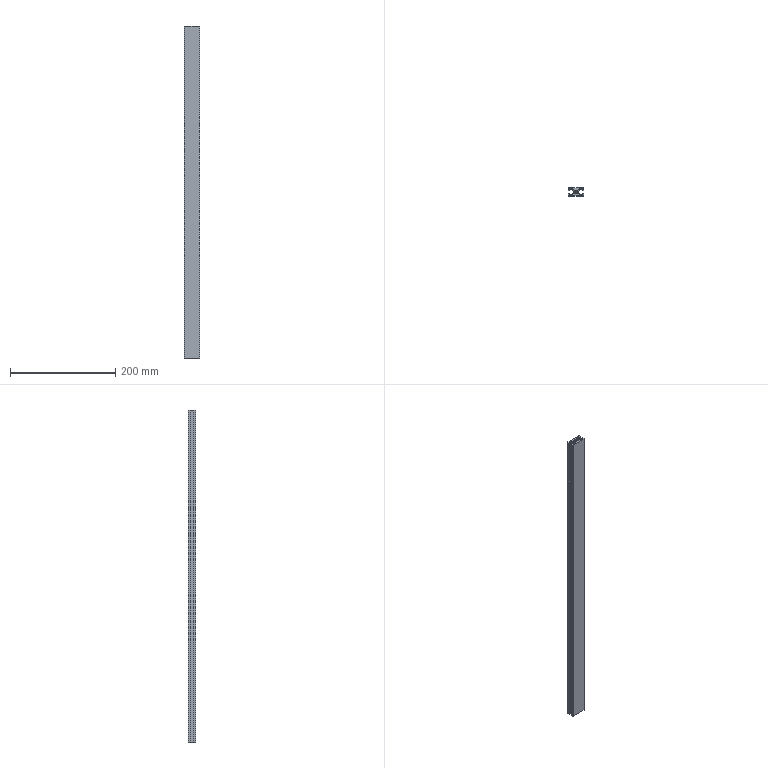Part | SolidWorks | features BaseBody 1, MoveFace 1 | 1 solid | 53 faces | box 30 x 15 x 630 mm | volume 151936 mm3 | plane 38 | cylinder 15 | commonest cylinder face diameters 1 x6 5 x5 2 x4